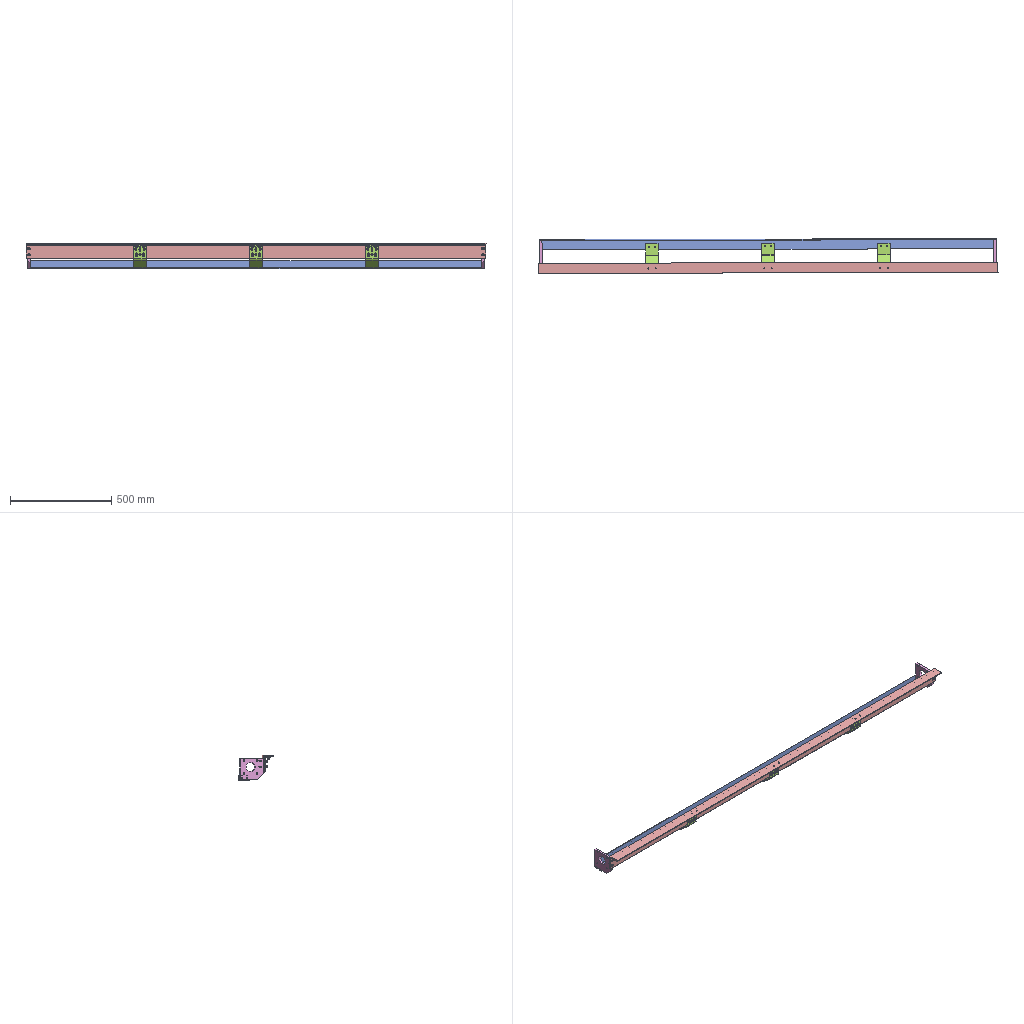Assembly | SolidWorks | 6 different items | 41 placed | box 2276 x 172 x 126 mm
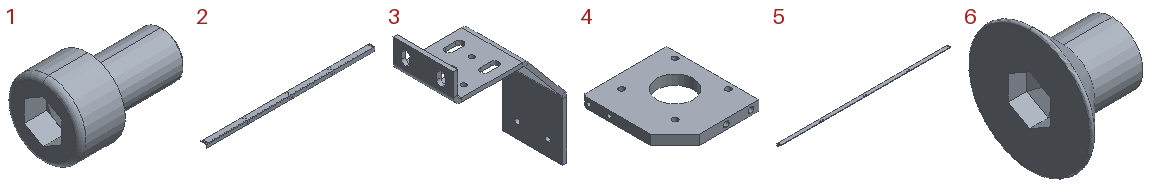Parts list (item | quantity | size | volume | features):
1 | x24 | 16 x 10 x 10 mm | 675.346 mm3 | features Fillet 2, RevCut 2, Boss 1, Chamfer 1, Cut 1, Extrusion 1, LPattern 1
2 | x1 | 2276 x 75 x 50 mm | 1389503 mm3 | features HoleWzd 2, Cut 1, WeldMemberFeat 1, WeldmentFeature 1
3 | x3 | 112.169 x 60 x 134.193 mm | 48668 mm3 | features EdgeFlange 3, HoleWzd 2, ICE 2, FlatPattern 1, SMBaseFlange 1, SheetMetal 1
4 | x2 | 103 x 112.5 x 12 mm | 110488 mm3 | features HoleWzd 3, Chamfer 2, ICE 2, 3DProfileFeature 1, Extrusion 1
5 | x1 | 2260 x 50 x 40 mm | 891378 mm3 | features Extrusion 1, HoleWzd 1, ICE 1, WeldmentFeature 1
6 | x10 | 8 x 12.034 x 12.034 mm | 331.77 mm3 | features Cut 3, Boss 1, Extrusion 1, Fillet 1, LPattern 1, RevCut 1
Mates (type | each side: item.copy, entity, surface, feature):
Coincident | 5.1 face plane Boss-Extrude1 | 3.1 face plane Edge-Flange3
Parallel | 2.1 face plane Unequal angle 7.5-5-5(1) | 3.1 face plane Base-Flange1
Parallel | 2.1 face plane Unequal angle 7.5-5-5(1) | 3.1 face plane Edge-Flange1
Coincident | 2.1 face plane Unequal angle 7.5-5-5(1) | 4.1 face plane Boss-Extrude1
Coincident | 2.1 face plane Unequal angle 7.5-5-5(1) | 4.2 face plane Boss-Extrude1
Coincident | 5.1 face plane Boss-Extrude1 | 4.2 face plane Boss-Extrude1 | 2 times
DistanceDim | 3.2 face plane Edge-Flange1 | 3.1 face plane Edge-Flange1
Coincident | 5.1 face plane Boss-Extrude1 | 4.1 face plane Boss-Extrude1 | 2 times
Coincident | 5.1 face plane Boss-Extrude2 | 4.2 face plane Boss-Extrude2
Coincident | 3.2 face plane Base-Flange1 | 1.1 face plane BaseHead
DistanceDim | 4.2 face plane Boss-Extrude1 | 2.1 face plane Unequal angle 7.5-5-5(1)
Coincident | 5.1 face plane Boss-Extrude1 | 3.3 face plane Edge-Flange3
DistanceDim | 3.2 face plane Edge-Flange2 | 4.1 face plane Boss-Extrude1
DistanceDim | 3.3 face plane Base-Flange1 | 3.2 face plane Base-Flange1
DistanceDim | 3.1 face plane Edge-Flange2 | 3.3 face plane Edge-Flange2
DistanceDim | 3.3 face plane Base-Flange1 | 3.1 face plane Base-Flange1
DistanceDim | 3.2 face plane Base-Flange1 | 3.1 face plane Base-Flange1
DistanceDim | 3.1 face plane Base-Flange1 | 2.1 face plane Unequal angle 7.5-5-5(1)
Coincident | 5.1 face cone CSK for M6 Hexagon lobular socket raised CTSK head screws1 | 6.1 face cone BaseHead
Coincident | 5.1 face cone CSK for M6 Hexagon lobular socket raised CTSK head screws1 | 6.2 face cone BaseHead
Coincident | 5.1 face cone CSK for M6 Hexagon lobular socket raised CTSK head screws1 | 6.3 face cone BaseHead
Coincident | 5.1 face cone CSK for M6 Hexagon lobular socket raised CTSK head screws1 | 6.4 face cone BaseHead
Coincident | 5.1 face cone CSK for M6 Hexagon lobular socket raised CTSK head screws1 | 6.5 face cone BaseHead
Coincident | 5.1 face cone CSK for M6 Hexagon lobular socket raised CTSK head screws1 | 6.6 face cone BaseHead
Coincident | 5.1 face cone CSK for M6 Hexagon lobular socket raised CTSK head screws1 | 6.7 face cone BaseHead
Coincident | 5.1 face cone CSK for M6 Hexagon lobular socket raised CTSK head screws1 | 6.8 face cone BaseHead
Coincident | 5.1 face cone CSK for M6 Hexagon lobular socket raised CTSK head screws1 | 6.9 face cone BaseHead
Coincident | 5.1 face cone CSK for M6 Hexagon lobular socket raised CTSK head screws1 | 6.10 face cone BaseHead
Concentric | 1.1 face cylinder BaseBody | 3.2 face cylinder M6 Tapped Hole3
Concentric | 1.2 face cylinder BaseBody | 3.2 face cylinder M6 Tapped Hole3
Concentric | 1.3 face cylinder BaseBody | 3.2 face cylinder M6 Tapped Hole3
Concentric | 3.3 face cylinder M6 Tapped Hole3 | 1.4 face cylinder BaseBody
Coincident | 3.3 face plane Base-Flange1 | 1.4 face plane BaseHead
Concentric | 3.3 face cylinder M6 Tapped Hole3 | 1.5 face cylinder BaseBody
Concentric | 3.3 face cylinder M6 Tapped Hole3 | 1.6 face cylinder BaseBody
Concentric | 3.1 face cylinder M6 Tapped Hole3 | 1.7 face cylinder BaseBody
Coincident | 3.1 face plane Base-Flange1 | 1.7 face plane BaseHead
Concentric | 3.1 edge | 1.8 face cylinder BaseBody
Concentric | 3.1 face cylinder M6 Tapped Hole3 | 1.9 face cylinder BaseBody
Coincident | 3.2 face plane Edge-Flange1 | 1.10 face plane BaseHead
Coincident | 3.2 face plane Edge-Flange1 | 1.11 face plane BaseHead
Coincident | 3.2 face plane Base-Flange1 | 1.12 face plane BaseHead
Coincident | 3.2 face plane Base-Flange1 | 1.13 face plane BaseHead
Coincident | 3.2 face plane Base-Flange1 | 1.14 face plane BaseHead
Coincident | 3.3 face plane Edge-Flange1 | 1.15 face plane BaseHead
Coincident | 3.3 face plane Edge-Flange1 | 1.16 face plane BaseHead
Coincident | 3.3 face plane Base-Flange1 | 1.17 face plane BaseHead
Coincident | 3.3 face plane Base-Flange1 | 1.18 face plane BaseHead
Coincident | 3.3 face plane Base-Flange1 | 1.19 face plane BaseHead
Coincident | 3.1 face plane Base-Flange1 | 1.20 face plane BaseHead
Coincident | 3.1 face plane Base-Flange1 | 1.21 face plane BaseHead
Coincident | 3.1 face plane Base-Flange1 | 1.22 face plane BaseHead
Coincident | 3.1 face plane Edge-Flange1 | 1.23 face plane BaseHead
Coincident | 3.1 face plane Edge-Flange1 | 1.24 face plane BaseHead
Concentric | 2.1 edge | 1.20 face cylinder BaseBody
Concentric | 2.1 face cylinder M6 Tapped Hole1 | 1.21 face cylinder BaseBody
Concentric | 2.1 face cylinder M6 Tapped Hole1 | 1.22 face cylinder BaseBody
Concentric | 2.1 face cylinder M6 Tapped Hole2 | 1.23 face cylinder BaseBody
Concentric | 2.1 face cylinder M6 Tapped Hole2 | 1.24 face cylinder BaseBody
Concentric | 2.1 face cylinder M6 Tapped Hole1 | 1.17 face cylinder BaseBody
Concentric | 2.1 face cylinder M6 Tapped Hole1 | 1.18 face cylinder BaseBody
Concentric | 2.1 face cylinder M6 Tapped Hole1 | 1.19 face cylinder BaseBody
Concentric | 2.1 face cylinder M6 Tapped Hole2 | 1.15 face cylinder BaseBody
Concentric | 2.1 face cylinder M6 Tapped Hole2 | 1.16 face cylinder BaseBody
Concentric | 2.1 face cylinder M6 Tapped Hole1 | 1.12 face cylinder BaseBody
Concentric | 2.1 face cylinder M6 Tapped Hole1 | 1.14 face cylinder BaseBody
Concentric | 2.1 face cylinder M6 Tapped Hole1 | 1.13 face cylinder BaseBody
Concentric | 2.1 face cylinder M6 Tapped Hole2 | 1.10 face cylinder BaseBody
Concentric | 2.1 face cylinder M6 Tapped Hole2 | 1.11 face cylinder BaseBody